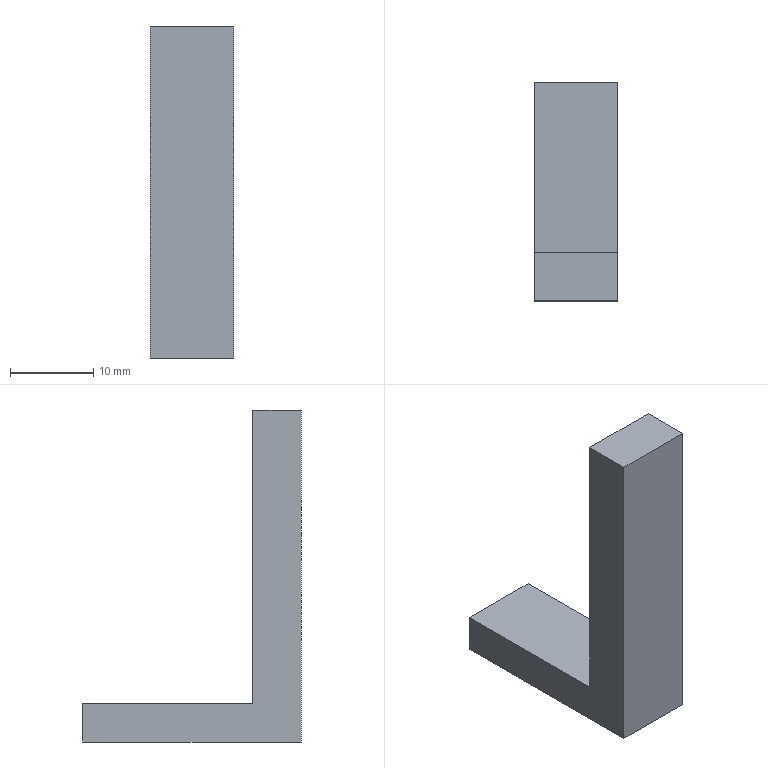Part | NX | features solid 2 | 1 solid | 8 faces | box 10 x 26.34 x 40 mm | volume 3290 mm3 | plane 8
STEP:
#1=CARTESIAN_POINT('',(2250.,260.94,-590.));
#2=VERTEX_POINT('',#1);
#3=CARTESIAN_POINT('',(2250.,234.6,-590.));
#4=VERTEX_POINT('',#3);
#5=CARTESIAN_POINT('',(2250.,260.94,-590.));
#6=CARTESIAN_POINT('',(2250.,252.16,-590.));
#7=CARTESIAN_POINT('',(2250.,243.38,-590.));
#8=CARTESIAN_POINT('',(2250.,234.6,-590.));
#9=B_SPLINE_CURVE_WITH_KNOTS('',3,(#5,#6,#7,#8),.UNSPECIFIED.,.F.,.F.,(4,4),(0.,0.1985),.PIECEWISE_BEZIER_KNOTS.);
#10=EDGE_CURVE('',#2,#4,#9,.T.);
#11=ORIENTED_EDGE('',*,*,#10,.F.);
#12=CARTESIAN_POINT('',(2260.,260.94,-590.));
#13=VERTEX_POINT('',#12);
#14=CARTESIAN_POINT('',(2260.,260.94,-590.));
#15=DIRECTION('',(-1.,0.,0.));
#16=VECTOR('',#15,1000.);
#17=LINE('',#14,#16);
#18=EDGE_CURVE('',#13,#2,#17,.T.);
#19=ORIENTED_EDGE('',*,*,#18,.F.);
#20=CARTESIAN_POINT('',(2260.,234.6,-590.));
#21=VERTEX_POINT('',#20);
#22=CARTESIAN_POINT('',(2260.,260.94,-590.));
#23=CARTESIAN_POINT('',(2260.,252.16,-590.));
#24=CARTESIAN_POINT('',(2260.,243.38,-590.));
#25=CARTESIAN_POINT('',(2260.,234.6,-590.));
#26=B_SPLINE_CURVE_WITH_KNOTS('',3,(#22,#23,#24,#25),.UNSPECIFIED.,.F.,.F.,(4,4),(0.,0.1985),.PIECEWISE_BEZIER_KNOTS.);
#27=EDGE_CURVE('',#13,#21,#26,.T.);
#28=ORIENTED_EDGE('',*,*,#27,.T.);
#29=CARTESIAN_POINT('',(2260.,234.6,-590.));
#30=DIRECTION('',(-1.,0.,0.));
#31=VECTOR('',#30,1000.);
#32=LINE('',#29,#31);
#33=EDGE_CURVE('',#21,#4,#32,.T.);
#34=ORIENTED_EDGE('',*,*,#33,.T.);
#35=EDGE_LOOP('',(#11,#19,#28,#34));
#36=FACE_BOUND('',#35,.T.);
#37=CARTESIAN_POINT('',(2260.,260.94,-590.));
#38=DIRECTION('',(0.,0.,-1.));
#39=DIRECTION('',(-1.,0.,0.));
#40=AXIS2_PLACEMENT_3D('',#37,#38,#39);
#41=PLANE('',#40);
#42=ADVANCED_FACE('',(#36),#41,.T.);
#43=CARTESIAN_POINT('',(2250.,234.6,-550.));
#44=VERTEX_POINT('',#43);
#45=CARTESIAN_POINT('',(2250.,234.6,-590.));
#46=CARTESIAN_POINT('',(2250.,234.6,-576.667));
#47=CARTESIAN_POINT('',(2250.,234.6,-563.333));
#48=CARTESIAN_POINT('',(2250.,234.6,-550.));
#49=B_SPLINE_CURVE_WITH_KNOTS('',3,(#45,#46,#47,#48),.UNSPECIFIED.,.F.,.F.,(4,4),(0.1985,0.5),.PIECEWISE_BEZIER_KNOTS.);
#50=EDGE_CURVE('',#4,#44,#49,.T.);
#51=ORIENTED_EDGE('',*,*,#50,.F.);
#52=ORIENTED_EDGE('',*,*,#33,.F.);
#53=CARTESIAN_POINT('',(2260.,234.6,-550.));
#54=VERTEX_POINT('',#53);
#55=CARTESIAN_POINT('',(2260.,234.6,-590.));
#56=CARTESIAN_POINT('',(2260.,234.6,-576.667));
#57=CARTESIAN_POINT('',(2260.,234.6,-563.333));
#58=CARTESIAN_POINT('',(2260.,234.6,-550.));
#59=B_SPLINE_CURVE_WITH_KNOTS('',3,(#55,#56,#57,#58),.UNSPECIFIED.,.F.,.F.,(4,4),(0.1985,0.5),.PIECEWISE_BEZIER_KNOTS.);
#60=EDGE_CURVE('',#21,#54,#59,.T.);
#61=ORIENTED_EDGE('',*,*,#60,.T.);
#62=CARTESIAN_POINT('',(2260.,234.6,-550.));
#63=DIRECTION('',(-1.,0.,0.));
#64=VECTOR('',#63,1000.);
#65=LINE('',#62,#64);
#66=EDGE_CURVE('',#54,#44,#65,.T.);
#67=ORIENTED_EDGE('',*,*,#66,.T.);
#68=EDGE_LOOP('',(#51,#52,#61,#67));
#69=FACE_BOUND('',#68,.T.);
#70=CARTESIAN_POINT('',(2260.,234.6,-590.));
#71=DIRECTION('',(0.,-1.,0.));
#72=DIRECTION('',(1.,0.,0.));
#73=AXIS2_PLACEMENT_3D('',#70,#71,#72);
#74=PLANE('',#73);
#75=ADVANCED_FACE('',(#69),#74,.T.);
#76=CARTESIAN_POINT('',(2250.,240.443,-550.));
#77=VERTEX_POINT('',#76);
#78=CARTESIAN_POINT('',(2250.,234.6,-550.));
#79=CARTESIAN_POINT('',(2250.,236.548,-550.));
#80=CARTESIAN_POINT('',(2250.,238.495,-550.));
#81=CARTESIAN_POINT('',(2250.,240.443,-550.));
#82=B_SPLINE_CURVE_WITH_KNOTS('',3,(#78,#79,#80,#81),.UNSPECIFIED.,.F.,.F.,(4,4),(0.5,0.544),.PIECEWISE_BEZIER_KNOTS.);
#83=EDGE_CURVE('',#44,#77,#82,.T.);
#84=ORIENTED_EDGE('',*,*,#83,.F.);
#85=ORIENTED_EDGE('',*,*,#66,.F.);
#86=CARTESIAN_POINT('',(2260.,240.443,-550.));
#87=VERTEX_POINT('',#86);
#88=CARTESIAN_POINT('',(2260.,234.6,-550.));
#89=CARTESIAN_POINT('',(2260.,236.548,-550.));
#90=CARTESIAN_POINT('',(2260.,238.495,-550.));
#91=CARTESIAN_POINT('',(2260.,240.443,-550.));
#92=B_SPLINE_CURVE_WITH_KNOTS('',3,(#88,#89,#90,#91),.UNSPECIFIED.,.F.,.F.,(4,4),(0.5,0.544),.PIECEWISE_BEZIER_KNOTS.);
#93=EDGE_CURVE('',#54,#87,#92,.T.);
#94=ORIENTED_EDGE('',*,*,#93,.T.);
#95=CARTESIAN_POINT('',(2260.,240.443,-550.));
#96=DIRECTION('',(-1.,0.,0.));
#97=VECTOR('',#96,1000.);
#98=LINE('',#95,#97);
#99=EDGE_CURVE('',#87,#77,#98,.T.);
#100=ORIENTED_EDGE('',*,*,#99,.T.);
#101=EDGE_LOOP('',(#84,#85,#94,#100));
#102=FACE_BOUND('',#101,.T.);
#103=CARTESIAN_POINT('',(2260.,234.6,-550.));
#104=DIRECTION('',(0.,0.,1.));
#105=DIRECTION('',(1.,0.,0.));
#106=AXIS2_PLACEMENT_3D('',#103,#104,#105);
#107=PLANE('',#106);
#108=ADVANCED_FACE('',(#102),#107,.T.);
#109=CARTESIAN_POINT('',(2250.,240.443,-585.35));
#110=VERTEX_POINT('',#109);
#111=CARTESIAN_POINT('',(2250.,240.443,-550.));
#112=CARTESIAN_POINT('',(2250.,240.443,-561.783));
#113=CARTESIAN_POINT('',(2250.,240.443,-573.567));
#114=CARTESIAN_POINT('',(2250.,240.443,-585.35));
#115=B_SPLINE_CURVE_WITH_KNOTS('',3,(#111,#112,#113,#114),.UNSPECIFIED.,.F.,.F.,(4,4),(0.544,0.8105),.PIECEWISE_BEZIER_KNOTS.);
#116=EDGE_CURVE('',#77,#110,#115,.T.);
#117=ORIENTED_EDGE('',*,*,#116,.F.);
#118=ORIENTED_EDGE('',*,*,#99,.F.);
#119=CARTESIAN_POINT('',(2260.,240.443,-585.35));
#120=VERTEX_POINT('',#119);
#121=CARTESIAN_POINT('',(2260.,240.443,-550.));
#122=CARTESIAN_POINT('',(2260.,240.443,-561.783));
#123=CARTESIAN_POINT('',(2260.,240.443,-573.567));
#124=CARTESIAN_POINT('',(2260.,240.443,-585.35));
#125=B_SPLINE_CURVE_WITH_KNOTS('',3,(#121,#122,#123,#124),.UNSPECIFIED.,.F.,.F.,(4,4),(0.544,0.8105),.PIECEWISE_BEZIER_KNOTS.);
#126=EDGE_CURVE('',#87,#120,#125,.T.);
#127=ORIENTED_EDGE('',*,*,#126,.T.);
#128=CARTESIAN_POINT('',(2260.,240.443,-585.35));
#129=DIRECTION('',(-1.,0.,0.));
#130=VECTOR('',#129,1000.);
#131=LINE('',#128,#130);
#132=EDGE_CURVE('',#120,#110,#131,.T.);
#133=ORIENTED_EDGE('',*,*,#132,.T.);
#134=EDGE_LOOP('',(#117,#118,#127,#133));
#135=FACE_BOUND('',#134,.T.);
#136=CARTESIAN_POINT('',(2260.,240.443,-550.));
#137=DIRECTION('',(0.,1.,0.));
#138=DIRECTION('',(-1.,0.,0.));
#139=AXIS2_PLACEMENT_3D('',#136,#137,#138);
#140=PLANE('',#139);
#141=ADVANCED_FACE('',(#135),#140,.T.);
#142=CARTESIAN_POINT('',(2250.,260.94,-585.35));
#143=VERTEX_POINT('',#142);
#144=CARTESIAN_POINT('',(2250.,240.443,-585.35));
#145=CARTESIAN_POINT('',(2250.,247.276,-585.35));
#146=CARTESIAN_POINT('',(2250.,254.108,-585.35));
#147=CARTESIAN_POINT('',(2250.,260.94,-585.35));
#148=B_SPLINE_CURVE_WITH_KNOTS('',3,(#144,#145,#146,#147),.UNSPECIFIED.,.F.,.F.,(4,4),(0.8105,0.965),.PIECEWISE_BEZIER_KNOTS.);
#149=EDGE_CURVE('',#110,#143,#148,.T.);
#150=ORIENTED_EDGE('',*,*,#149,.F.);
#151=ORIENTED_EDGE('',*,*,#132,.F.);
#152=CARTESIAN_POINT('',(2260.,260.94,-585.35));
#153=VERTEX_POINT('',#152);
#154=CARTESIAN_POINT('',(2260.,240.443,-585.35));
#155=CARTESIAN_POINT('',(2260.,247.276,-585.35));
#156=CARTESIAN_POINT('',(2260.,254.108,-585.35));
#157=CARTESIAN_POINT('',(2260.,260.94,-585.35));
#158=B_SPLINE_CURVE_WITH_KNOTS('',3,(#154,#155,#156,#157),.UNSPECIFIED.,.F.,.F.,(4,4),(0.8105,0.965),.PIECEWISE_BEZIER_KNOTS.);
#159=EDGE_CURVE('',#120,#153,#158,.T.);
#160=ORIENTED_EDGE('',*,*,#159,.T.);
#161=CARTESIAN_POINT('',(2260.,260.94,-585.35));
#162=DIRECTION('',(-1.,0.,0.));
#163=VECTOR('',#162,1000.);
#164=LINE('',#161,#163);
#165=EDGE_CURVE('',#153,#143,#164,.T.);
#166=ORIENTED_EDGE('',*,*,#165,.T.);
#167=EDGE_LOOP('',(#150,#151,#160,#166));
#168=FACE_BOUND('',#167,.T.);
#169=CARTESIAN_POINT('',(2260.,240.443,-585.35));
#170=DIRECTION('',(0.,0.,1.));
#171=DIRECTION('',(1.,0.,0.));
#172=AXIS2_PLACEMENT_3D('',#169,#170,#171);
#173=PLANE('',#172);
#174=ADVANCED_FACE('',(#168),#173,.T.);
#175=CARTESIAN_POINT('',(2250.,260.94,-585.35));
#176=CARTESIAN_POINT('',(2250.,260.94,-586.9));
#177=CARTESIAN_POINT('',(2250.,260.94,-588.45));
#178=CARTESIAN_POINT('',(2250.,260.94,-590.));
#179=B_SPLINE_CURVE_WITH_KNOTS('',3,(#175,#176,#177,#178),.UNSPECIFIED.,.F.,.F.,(4,4),(0.965,1.),.PIECEWISE_BEZIER_KNOTS.);
#180=EDGE_CURVE('',#143,#2,#179,.T.);
#181=ORIENTED_EDGE('',*,*,#180,.F.);
#182=ORIENTED_EDGE('',*,*,#165,.F.);
#183=CARTESIAN_POINT('',(2260.,260.94,-585.35));
#184=CARTESIAN_POINT('',(2260.,260.94,-586.9));
#185=CARTESIAN_POINT('',(2260.,260.94,-588.45));
#186=CARTESIAN_POINT('',(2260.,260.94,-590.));
#187=B_SPLINE_CURVE_WITH_KNOTS('',3,(#183,#184,#185,#186),.UNSPECIFIED.,.F.,.F.,(4,4),(0.965,1.),.PIECEWISE_BEZIER_KNOTS.);
#188=EDGE_CURVE('',#153,#13,#187,.T.);
#189=ORIENTED_EDGE('',*,*,#188,.T.);
#190=ORIENTED_EDGE('',*,*,#18,.T.);
#191=EDGE_LOOP('',(#181,#182,#189,#190));
#192=FACE_BOUND('',#191,.T.);
#193=CARTESIAN_POINT('',(2260.,260.94,-585.35));
#194=DIRECTION('',(0.,1.,0.));
#195=DIRECTION('',(-1.,0.,0.));
#196=AXIS2_PLACEMENT_3D('',#193,#194,#195);
#197=PLANE('',#196);
#198=ADVANCED_FACE('',(#192),#197,.T.);
#199=ORIENTED_EDGE('',*,*,#27,.F.);
#200=ORIENTED_EDGE('',*,*,#188,.F.);
#201=ORIENTED_EDGE('',*,*,#159,.F.);
#202=ORIENTED_EDGE('',*,*,#126,.F.);
#203=ORIENTED_EDGE('',*,*,#93,.F.);
#204=ORIENTED_EDGE('',*,*,#60,.F.);
#205=EDGE_LOOP('',(#199,#200,#201,#202,#203,#204));
#206=FACE_BOUND('',#205,.T.);
#207=CARTESIAN_POINT('',(2260.,247.77,-590.));
#208=DIRECTION('',(1.,0.,0.));
#209=DIRECTION('',(0.,1.,0.));
#210=AXIS2_PLACEMENT_3D('',#207,#208,#209);
#211=PLANE('',#210);
#212=ADVANCED_FACE('',(#206),#211,.T.);
#213=ORIENTED_EDGE('',*,*,#10,.T.);
#214=ORIENTED_EDGE('',*,*,#50,.T.);
#215=ORIENTED_EDGE('',*,*,#83,.T.);
#216=ORIENTED_EDGE('',*,*,#116,.T.);
#217=ORIENTED_EDGE('',*,*,#149,.T.);
#218=ORIENTED_EDGE('',*,*,#180,.T.);
#219=EDGE_LOOP('',(#213,#214,#215,#216,#217,#218));
#220=FACE_BOUND('',#219,.T.);
#221=CARTESIAN_POINT('',(2250.,247.77,-590.));
#222=DIRECTION('',(1.,0.,0.));
#223=DIRECTION('',(0.,1.,0.));
#224=AXIS2_PLACEMENT_3D('',#221,#222,#223);
#225=PLANE('',#224);
#226=ADVANCED_FACE('',(#220),#225,.F.);
#227=CLOSED_SHELL('',(#42,#75,#108,#141,#174,#198,#212,#226));
#228=MANIFOLD_SOLID_BREP('',#227);
#229=(LENGTH_UNIT()NAMED_UNIT(*)SI_UNIT(.MILLI.,.METRE.));
#230=UNCERTAINTY_MEASURE_WITH_UNIT(LENGTH_MEASURE(0.00001),#229,'','');
#231=(NAMED_UNIT(*)PLANE_ANGLE_UNIT()SI_UNIT($,.RADIAN.));
#232=(NAMED_UNIT(*)SI_UNIT($,.STERADIAN.)SOLID_ANGLE_UNIT());
#233=(GEOMETRIC_REPRESENTATION_CONTEXT(3)GLOBAL_UNCERTAINTY_ASSIGNED_CONTEXT((#230))GLOBAL_UNIT_ASSIGNED_CONTEXT((#229,#231,#232))REPRESENTATION_CONTEXT('',''));
#234=ADVANCED_BREP_SHAPE_REPRESENTATION('',(#228),#233);